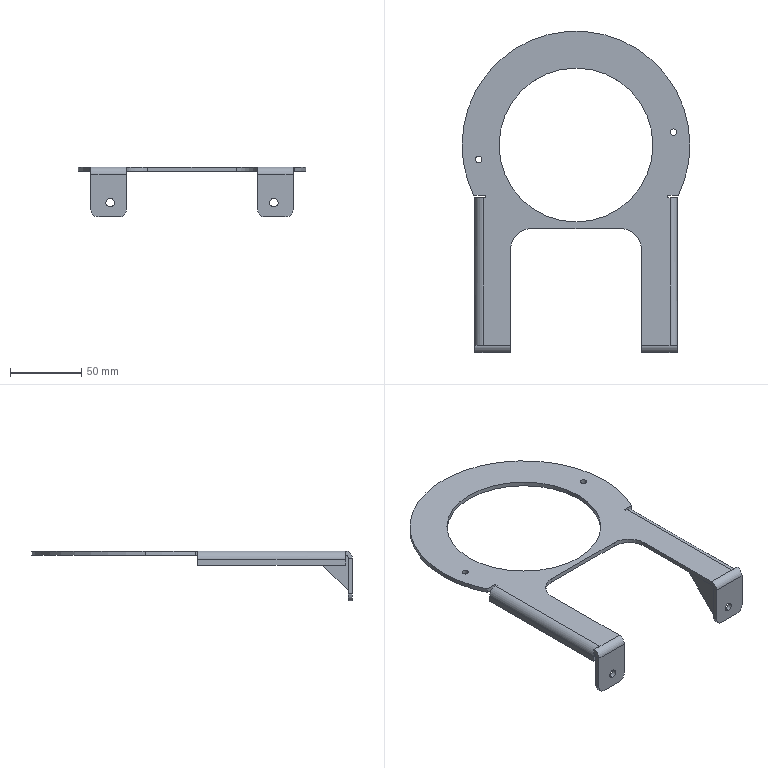Part | STEP file | Cup dropper fixing bracket V1.201001 | 3 solids | 78 faces | box 160 x 225.6 x 35 mm | volume 51040 mm3 | plane 51 | cylinder 27 | commonest cylinder face diameters 10 x7 6 x5 4.5 x4 4 x3 160 x3 30 x2